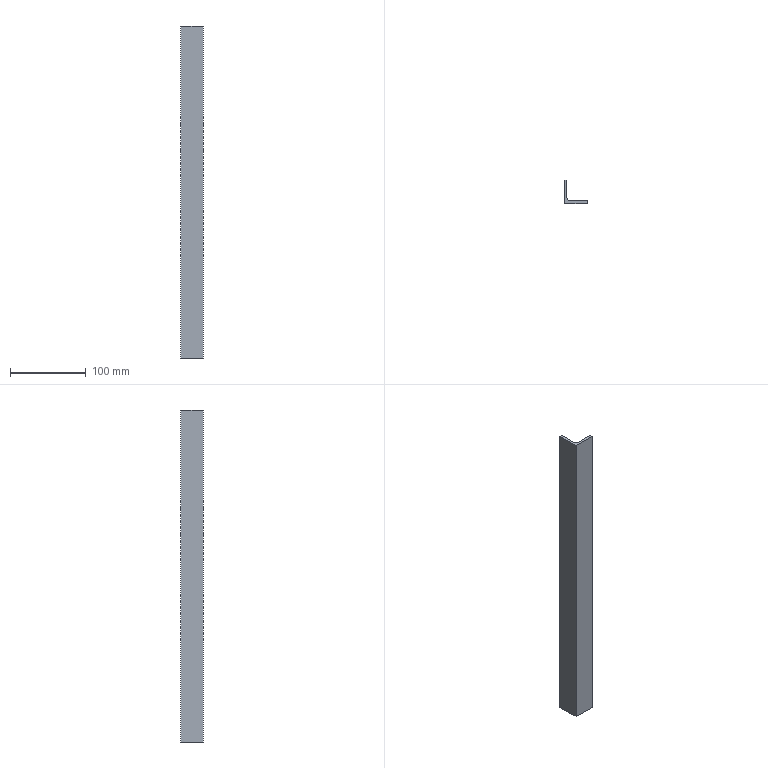Part | SolidWorks | features Extrusion 1 | 1 solid | 11 faces | box 30 x 30 x 438.8 mm | volume 76753 mm3 | plane 8 | cylinder 3 | commonest cylinder face diameters 2 x2 9 x1
STEP:
#1=CARTESIAN_POINT('',(2.,30.,-219.4));
#2=VERTEX_POINT('',#1);
#3=CARTESIAN_POINT('',(3.,29.,-219.4));
#4=VERTEX_POINT('',#3);
#5=CARTESIAN_POINT('',(2.,29.,-219.4));
#6=DIRECTION('',(0.,0.,-1.));
#7=DIRECTION('',(-1.,0.,0.));
#8=AXIS2_PLACEMENT_3D('',#5,#6,#7);
#9=CIRCLE('',#8,1.);
#10=EDGE_CURVE('',#2,#4,#9,.T.);
#11=ORIENTED_EDGE('',*,*,#10,.F.);
#12=CARTESIAN_POINT('',(2.,30.,219.4));
#13=VERTEX_POINT('',#12);
#14=CARTESIAN_POINT('',(2.,30.,219.4));
#15=DIRECTION('',(0.,0.,-1.));
#16=VECTOR('',#15,1000.);
#17=LINE('',#14,#16);
#18=EDGE_CURVE('',#13,#2,#17,.T.);
#19=ORIENTED_EDGE('',*,*,#18,.F.);
#20=CARTESIAN_POINT('',(3.,29.,219.4));
#21=VERTEX_POINT('',#20);
#22=CARTESIAN_POINT('',(2.,29.,219.4));
#23=DIRECTION('',(0.,0.,-1.));
#24=DIRECTION('',(-1.,0.,0.));
#25=AXIS2_PLACEMENT_3D('',#22,#23,#24);
#26=CIRCLE('',#25,1.);
#27=EDGE_CURVE('',#13,#21,#26,.T.);
#28=ORIENTED_EDGE('',*,*,#27,.T.);
#29=CARTESIAN_POINT('',(3.,29.,219.4));
#30=DIRECTION('',(0.,0.,-1.));
#31=VECTOR('',#30,1000.);
#32=LINE('',#29,#31);
#33=EDGE_CURVE('',#21,#4,#32,.T.);
#34=ORIENTED_EDGE('',*,*,#33,.T.);
#35=EDGE_LOOP('',(#11,#19,#28,#34));
#36=FACE_OUTER_BOUND('',#35,.T.);
#37=CARTESIAN_POINT('',(2.,29.,219.4));
#38=DIRECTION('',(0.,0.,-1.));
#39=DIRECTION('',(-1.,0.,0.));
#40=AXIS2_PLACEMENT_3D('',#37,#38,#39);
#41=CYLINDRICAL_SURFACE('',#40,1.);
#42=ADVANCED_FACE('',(#36),#41,.T.);
#43=CARTESIAN_POINT('',(0.,30.,-219.4));
#44=VERTEX_POINT('',#43);
#45=CARTESIAN_POINT('',(0.,30.,-219.4));
#46=DIRECTION('',(1.,0.,0.));
#47=VECTOR('',#46,1000.);
#48=LINE('',#45,#47);
#49=EDGE_CURVE('',#44,#2,#48,.T.);
#50=ORIENTED_EDGE('',*,*,#49,.F.);
#51=CARTESIAN_POINT('',(0.,30.,219.4));
#52=VERTEX_POINT('',#51);
#53=CARTESIAN_POINT('',(0.,30.,219.4));
#54=DIRECTION('',(0.,0.,-1.));
#55=VECTOR('',#54,1000.);
#56=LINE('',#53,#55);
#57=EDGE_CURVE('',#52,#44,#56,.T.);
#58=ORIENTED_EDGE('',*,*,#57,.F.);
#59=CARTESIAN_POINT('',(0.,30.,219.4));
#60=DIRECTION('',(1.,0.,0.));
#61=VECTOR('',#60,1000.);
#62=LINE('',#59,#61);
#63=EDGE_CURVE('',#52,#13,#62,.T.);
#64=ORIENTED_EDGE('',*,*,#63,.T.);
#65=ORIENTED_EDGE('',*,*,#18,.T.);
#66=EDGE_LOOP('',(#50,#58,#64,#65));
#67=FACE_OUTER_BOUND('',#66,.T.);
#68=CARTESIAN_POINT('',(0.,30.,219.4));
#69=DIRECTION('',(0.,1.,0.));
#70=DIRECTION('',(0.,0.,1.));
#71=AXIS2_PLACEMENT_3D('',#68,#69,#70);
#72=PLANE('',#71);
#73=ADVANCED_FACE('',(#67),#72,.T.);
#74=CARTESIAN_POINT('',(0.,0.,-219.4));
#75=VERTEX_POINT('',#74);
#76=CARTESIAN_POINT('',(0.,0.,-219.4));
#77=DIRECTION('',(0.,1.,0.));
#78=VECTOR('',#77,1000.);
#79=LINE('',#76,#78);
#80=EDGE_CURVE('',#75,#44,#79,.T.);
#81=ORIENTED_EDGE('',*,*,#80,.F.);
#82=CARTESIAN_POINT('',(0.,0.,219.4));
#83=VERTEX_POINT('',#82);
#84=CARTESIAN_POINT('',(0.,0.,219.4));
#85=DIRECTION('',(0.,0.,-1.));
#86=VECTOR('',#85,1000.);
#87=LINE('',#84,#86);
#88=EDGE_CURVE('',#83,#75,#87,.T.);
#89=ORIENTED_EDGE('',*,*,#88,.F.);
#90=CARTESIAN_POINT('',(0.,0.,219.4));
#91=DIRECTION('',(0.,1.,0.));
#92=VECTOR('',#91,1000.);
#93=LINE('',#90,#92);
#94=EDGE_CURVE('',#83,#52,#93,.T.);
#95=ORIENTED_EDGE('',*,*,#94,.T.);
#96=ORIENTED_EDGE('',*,*,#57,.T.);
#97=EDGE_LOOP('',(#81,#89,#95,#96));
#98=FACE_OUTER_BOUND('',#97,.T.);
#99=CARTESIAN_POINT('',(0.,0.,219.4));
#100=DIRECTION('',(-1.,0.,0.));
#101=DIRECTION('',(0.,0.,1.));
#102=AXIS2_PLACEMENT_3D('',#99,#100,#101);
#103=PLANE('',#102);
#104=ADVANCED_FACE('',(#98),#103,.T.);
#105=CARTESIAN_POINT('',(30.,0.,-219.4));
#106=VERTEX_POINT('',#105);
#107=CARTESIAN_POINT('',(30.,0.,-219.4));
#108=DIRECTION('',(-1.,0.,0.));
#109=VECTOR('',#108,1000.);
#110=LINE('',#107,#109);
#111=EDGE_CURVE('',#106,#75,#110,.T.);
#112=ORIENTED_EDGE('',*,*,#111,.F.);
#113=CARTESIAN_POINT('',(30.,0.,219.4));
#114=VERTEX_POINT('',#113);
#115=CARTESIAN_POINT('',(30.,0.,219.4));
#116=DIRECTION('',(0.,0.,-1.));
#117=VECTOR('',#116,1000.);
#118=LINE('',#115,#117);
#119=EDGE_CURVE('',#114,#106,#118,.T.);
#120=ORIENTED_EDGE('',*,*,#119,.F.);
#121=CARTESIAN_POINT('',(30.,0.,219.4));
#122=DIRECTION('',(-1.,0.,0.));
#123=VECTOR('',#122,1000.);
#124=LINE('',#121,#123);
#125=EDGE_CURVE('',#114,#83,#124,.T.);
#126=ORIENTED_EDGE('',*,*,#125,.T.);
#127=ORIENTED_EDGE('',*,*,#88,.T.);
#128=EDGE_LOOP('',(#112,#120,#126,#127));
#129=FACE_OUTER_BOUND('',#128,.T.);
#130=CARTESIAN_POINT('',(30.,0.,219.4));
#131=DIRECTION('',(0.,-1.,0.));
#132=DIRECTION('',(0.,0.,-1.));
#133=AXIS2_PLACEMENT_3D('',#130,#131,#132);
#134=PLANE('',#133);
#135=ADVANCED_FACE('',(#129),#134,.T.);
#136=CARTESIAN_POINT('',(30.,2.,-219.4));
#137=VERTEX_POINT('',#136);
#138=CARTESIAN_POINT('',(30.,0.,-219.4));
#139=DIRECTION('',(0.,1.,0.));
#140=VECTOR('',#139,1000.);
#141=LINE('',#138,#140);
#142=EDGE_CURVE('',#106,#137,#141,.T.);
#143=ORIENTED_EDGE('',*,*,#142,.T.);
#144=CARTESIAN_POINT('',(30.,2.,219.4));
#145=VERTEX_POINT('',#144);
#146=CARTESIAN_POINT('',(30.,2.,219.4));
#147=DIRECTION('',(0.,0.,-1.));
#148=VECTOR('',#147,1000.);
#149=LINE('',#146,#148);
#150=EDGE_CURVE('',#145,#137,#149,.T.);
#151=ORIENTED_EDGE('',*,*,#150,.F.);
#152=CARTESIAN_POINT('',(30.,0.,219.4));
#153=DIRECTION('',(0.,1.,0.));
#154=VECTOR('',#153,1000.);
#155=LINE('',#152,#154);
#156=EDGE_CURVE('',#114,#145,#155,.T.);
#157=ORIENTED_EDGE('',*,*,#156,.F.);
#158=ORIENTED_EDGE('',*,*,#119,.T.);
#159=EDGE_LOOP('',(#143,#151,#157,#158));
#160=FACE_OUTER_BOUND('',#159,.T.);
#161=CARTESIAN_POINT('',(30.,0.,219.4));
#162=DIRECTION('',(-1.,0.,0.));
#163=DIRECTION('',(0.,0.,1.));
#164=AXIS2_PLACEMENT_3D('',#161,#162,#163);
#165=PLANE('',#164);
#166=ADVANCED_FACE('',(#160),#165,.F.);
#167=CARTESIAN_POINT('',(29.,3.,-219.4));
#168=VERTEX_POINT('',#167);
#169=CARTESIAN_POINT('',(29.,2.,-219.4));
#170=DIRECTION('',(0.,0.,1.));
#171=DIRECTION('',(1.,0.,0.));
#172=AXIS2_PLACEMENT_3D('',#169,#170,#171);
#173=CIRCLE('',#172,1.);
#174=EDGE_CURVE('',#137,#168,#173,.T.);
#175=ORIENTED_EDGE('',*,*,#174,.T.);
#176=CARTESIAN_POINT('',(29.,3.,219.4));
#177=VERTEX_POINT('',#176);
#178=CARTESIAN_POINT('',(29.,3.,219.4));
#179=DIRECTION('',(0.,0.,-1.));
#180=VECTOR('',#179,1000.);
#181=LINE('',#178,#180);
#182=EDGE_CURVE('',#177,#168,#181,.T.);
#183=ORIENTED_EDGE('',*,*,#182,.F.);
#184=CARTESIAN_POINT('',(29.,2.,219.4));
#185=DIRECTION('',(0.,0.,1.));
#186=DIRECTION('',(1.,0.,0.));
#187=AXIS2_PLACEMENT_3D('',#184,#185,#186);
#188=CIRCLE('',#187,1.);
#189=EDGE_CURVE('',#145,#177,#188,.T.);
#190=ORIENTED_EDGE('',*,*,#189,.F.);
#191=ORIENTED_EDGE('',*,*,#150,.T.);
#192=EDGE_LOOP('',(#175,#183,#190,#191));
#193=FACE_OUTER_BOUND('',#192,.T.);
#194=CARTESIAN_POINT('',(29.,2.,219.4));
#195=DIRECTION('',(0.,0.,-1.));
#196=DIRECTION('',(-1.,0.,0.));
#197=AXIS2_PLACEMENT_3D('',#194,#195,#196);
#198=CYLINDRICAL_SURFACE('',#197,1.);
#199=ADVANCED_FACE('',(#193),#198,.T.);
#200=CARTESIAN_POINT('',(7.5,3.,-219.4));
#201=VERTEX_POINT('',#200);
#202=CARTESIAN_POINT('',(7.5,3.,-219.4));
#203=DIRECTION('',(1.,0.,0.));
#204=VECTOR('',#203,1000.);
#205=LINE('',#202,#204);
#206=EDGE_CURVE('',#201,#168,#205,.T.);
#207=ORIENTED_EDGE('',*,*,#206,.F.);
#208=CARTESIAN_POINT('',(7.5,3.,219.4));
#209=VERTEX_POINT('',#208);
#210=CARTESIAN_POINT('',(7.5,3.,219.4));
#211=DIRECTION('',(0.,0.,-1.));
#212=VECTOR('',#211,1000.);
#213=LINE('',#210,#212);
#214=EDGE_CURVE('',#209,#201,#213,.T.);
#215=ORIENTED_EDGE('',*,*,#214,.F.);
#216=CARTESIAN_POINT('',(7.5,3.,219.4));
#217=DIRECTION('',(1.,0.,0.));
#218=VECTOR('',#217,1000.);
#219=LINE('',#216,#218);
#220=EDGE_CURVE('',#209,#177,#219,.T.);
#221=ORIENTED_EDGE('',*,*,#220,.T.);
#222=ORIENTED_EDGE('',*,*,#182,.T.);
#223=EDGE_LOOP('',(#207,#215,#221,#222));
#224=FACE_OUTER_BOUND('',#223,.T.);
#225=CARTESIAN_POINT('',(7.5,3.,219.4));
#226=DIRECTION('',(0.,1.,0.));
#227=DIRECTION('',(-1.,0.,0.));
#228=AXIS2_PLACEMENT_3D('',#225,#226,#227);
#229=PLANE('',#228);
#230=ADVANCED_FACE('',(#224),#229,.T.);
#231=CARTESIAN_POINT('',(3.,7.5,-219.4));
#232=VERTEX_POINT('',#231);
#233=CARTESIAN_POINT('',(7.5,7.5,-219.4));
#234=DIRECTION('',(0.,0.,-1.));
#235=DIRECTION('',(-1.,0.,0.));
#236=AXIS2_PLACEMENT_3D('',#233,#234,#235);
#237=CIRCLE('',#236,4.5);
#238=EDGE_CURVE('',#201,#232,#237,.T.);
#239=ORIENTED_EDGE('',*,*,#238,.T.);
#240=CARTESIAN_POINT('',(3.,7.5,219.4));
#241=VERTEX_POINT('',#240);
#242=CARTESIAN_POINT('',(3.,7.5,219.4));
#243=DIRECTION('',(0.,0.,-1.));
#244=VECTOR('',#243,1000.);
#245=LINE('',#242,#244);
#246=EDGE_CURVE('',#241,#232,#245,.T.);
#247=ORIENTED_EDGE('',*,*,#246,.F.);
#248=CARTESIAN_POINT('',(7.5,7.5,219.4));
#249=DIRECTION('',(0.,0.,-1.));
#250=DIRECTION('',(-1.,0.,0.));
#251=AXIS2_PLACEMENT_3D('',#248,#249,#250);
#252=CIRCLE('',#251,4.5);
#253=EDGE_CURVE('',#209,#241,#252,.T.);
#254=ORIENTED_EDGE('',*,*,#253,.F.);
#255=ORIENTED_EDGE('',*,*,#214,.T.);
#256=EDGE_LOOP('',(#239,#247,#254,#255));
#257=FACE_OUTER_BOUND('',#256,.T.);
#258=CARTESIAN_POINT('',(7.5,7.5,219.4));
#259=DIRECTION('',(0.,0.,-1.));
#260=DIRECTION('',(-1.,0.,0.));
#261=AXIS2_PLACEMENT_3D('',#258,#259,#260);
#262=CYLINDRICAL_SURFACE('',#261,4.5);
#263=ADVANCED_FACE('',(#257),#262,.F.);
#264=CARTESIAN_POINT('',(3.,29.,-219.4));
#265=DIRECTION('',(0.,-1.,0.));
#266=VECTOR('',#265,1000.);
#267=LINE('',#264,#266);
#268=EDGE_CURVE('',#4,#232,#267,.T.);
#269=ORIENTED_EDGE('',*,*,#268,.F.);
#270=ORIENTED_EDGE('',*,*,#33,.F.);
#271=CARTESIAN_POINT('',(3.,29.,219.4));
#272=DIRECTION('',(0.,-1.,0.));
#273=VECTOR('',#272,1000.);
#274=LINE('',#271,#273);
#275=EDGE_CURVE('',#21,#241,#274,.T.);
#276=ORIENTED_EDGE('',*,*,#275,.T.);
#277=ORIENTED_EDGE('',*,*,#246,.T.);
#278=EDGE_LOOP('',(#269,#270,#276,#277));
#279=FACE_OUTER_BOUND('',#278,.T.);
#280=CARTESIAN_POINT('',(3.,29.,219.4));
#281=DIRECTION('',(1.,0.,0.));
#282=DIRECTION('',(0.,1.,0.));
#283=AXIS2_PLACEMENT_3D('',#280,#281,#282);
#284=PLANE('',#283);
#285=ADVANCED_FACE('',(#279),#284,.T.);
#286=ORIENTED_EDGE('',*,*,#27,.F.);
#287=ORIENTED_EDGE('',*,*,#63,.F.);
#288=ORIENTED_EDGE('',*,*,#94,.F.);
#289=ORIENTED_EDGE('',*,*,#125,.F.);
#290=ORIENTED_EDGE('',*,*,#156,.T.);
#291=ORIENTED_EDGE('',*,*,#189,.T.);
#292=ORIENTED_EDGE('',*,*,#220,.F.);
#293=ORIENTED_EDGE('',*,*,#253,.T.);
#294=ORIENTED_EDGE('',*,*,#275,.F.);
#295=EDGE_LOOP('',(#286,#287,#288,#289,#290,#291,#292,#293,#294));
#296=FACE_OUTER_BOUND('',#295,.T.);
#297=CARTESIAN_POINT('',(2.,29.,219.4));
#298=DIRECTION('',(0.,0.,-1.));
#299=DIRECTION('',(-1.,0.,0.));
#300=AXIS2_PLACEMENT_3D('',#297,#298,#299);
#301=PLANE('',#300);
#302=ADVANCED_FACE('',(#296),#301,.F.);
#303=ORIENTED_EDGE('',*,*,#10,.T.);
#304=ORIENTED_EDGE('',*,*,#268,.T.);
#305=ORIENTED_EDGE('',*,*,#238,.F.);
#306=ORIENTED_EDGE('',*,*,#206,.T.);
#307=ORIENTED_EDGE('',*,*,#174,.F.);
#308=ORIENTED_EDGE('',*,*,#142,.F.);
#309=ORIENTED_EDGE('',*,*,#111,.T.);
#310=ORIENTED_EDGE('',*,*,#80,.T.);
#311=ORIENTED_EDGE('',*,*,#49,.T.);
#312=EDGE_LOOP('',(#303,#304,#305,#306,#307,#308,#309,#310,#311));
#313=FACE_OUTER_BOUND('',#312,.T.);
#314=CARTESIAN_POINT('',(2.,29.,-219.4));
#315=DIRECTION('',(0.,0.,-1.));
#316=DIRECTION('',(-1.,0.,0.));
#317=AXIS2_PLACEMENT_3D('',#314,#315,#316);
#318=PLANE('',#317);
#319=ADVANCED_FACE('',(#313),#318,.T.);
#320=CLOSED_SHELL('',(#42,#73,#104,#135,#166,#199,#230,#263,#285,#302,#319));
#321=MANIFOLD_SOLID_BREP('',#320);
#322=CARTESIAN_POINT('',(0.,0.,0.));
#323=DIRECTION('',(0.,0.,1.));
#324=DIRECTION('',(1.,0.,0.));
#325=AXIS2_PLACEMENT_3D('',#322,#323,#324);
#326=(LENGTH_UNIT()NAMED_UNIT(*)SI_UNIT(.MILLI.,.METRE.));
#327=UNCERTAINTY_MEASURE_WITH_UNIT(LENGTH_MEASURE(0.00001),#326,'','');
#328=(NAMED_UNIT(*)PLANE_ANGLE_UNIT()SI_UNIT($,.RADIAN.));
#329=(NAMED_UNIT(*)SI_UNIT($,.STERADIAN.)SOLID_ANGLE_UNIT());
#330=(GEOMETRIC_REPRESENTATION_CONTEXT(3)GLOBAL_UNCERTAINTY_ASSIGNED_CONTEXT((#327))GLOBAL_UNIT_ASSIGNED_CONTEXT((#326,#328,#329))REPRESENTATION_CONTEXT('',''));
#331=ADVANCED_BREP_SHAPE_REPRESENTATION('',(#321,#325),#330);